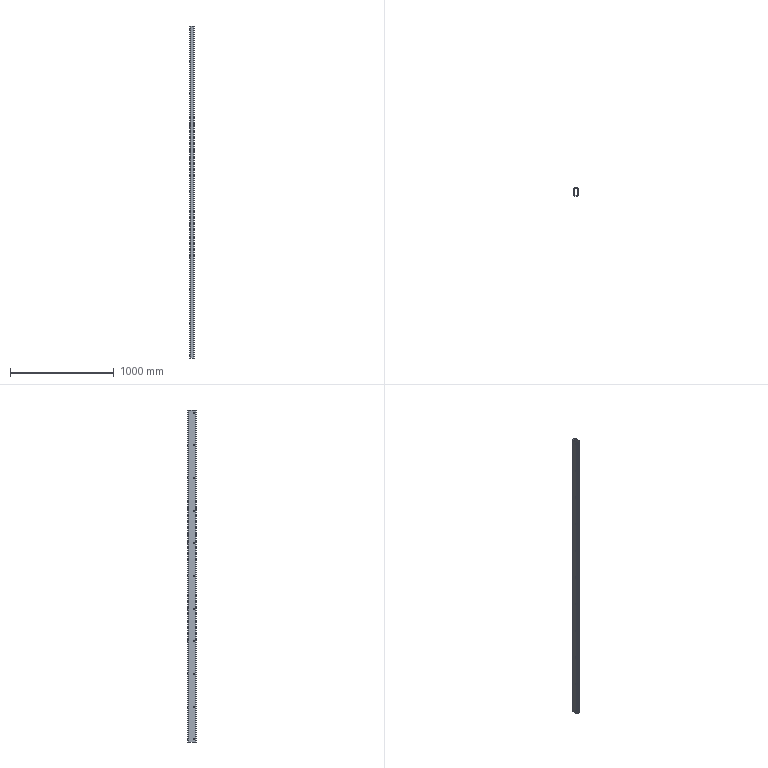Part | SolidWorks | features ICE 2, Extrusion 1, HoleWzd 1, LPattern 1 | 1 solid | 62 faces | box 40 x 80 x 3200 mm | volume 3306758 mm3 | cylinder 52 | plane 10 | commonest cylinder face diameters 6.8 x22 11 x22 10 x4 20 x4